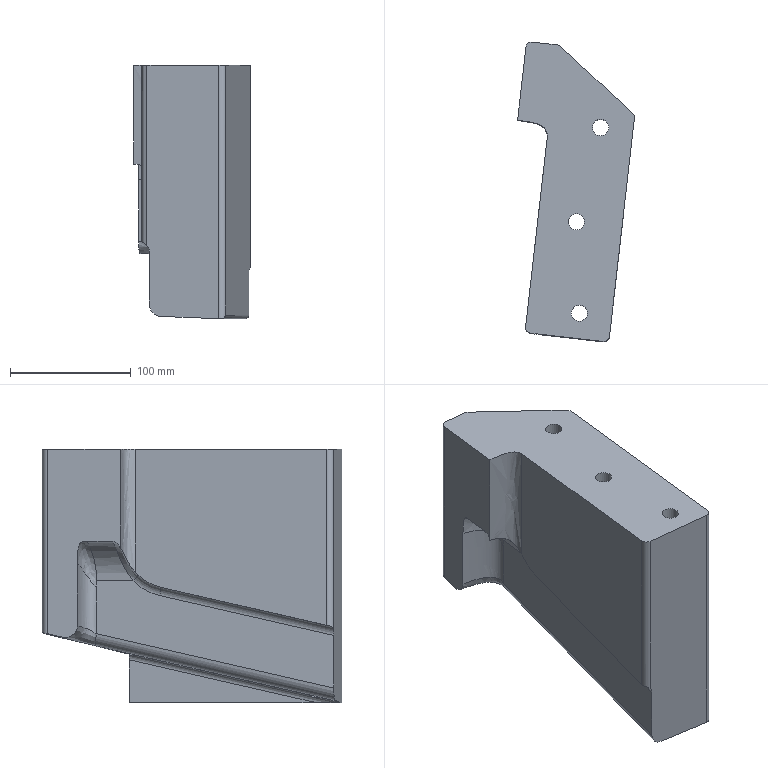Part | NX | features solid 2 | 1 solid | 43 faces | volume 2794841 mm3 | cylinder 19 | plane 16 | spline 5 | cone 2 | torus 1 | commonest cylinder face diameters 10 x6 20 x4 13.5 x3 8.5 x2 6 x1 14 x1